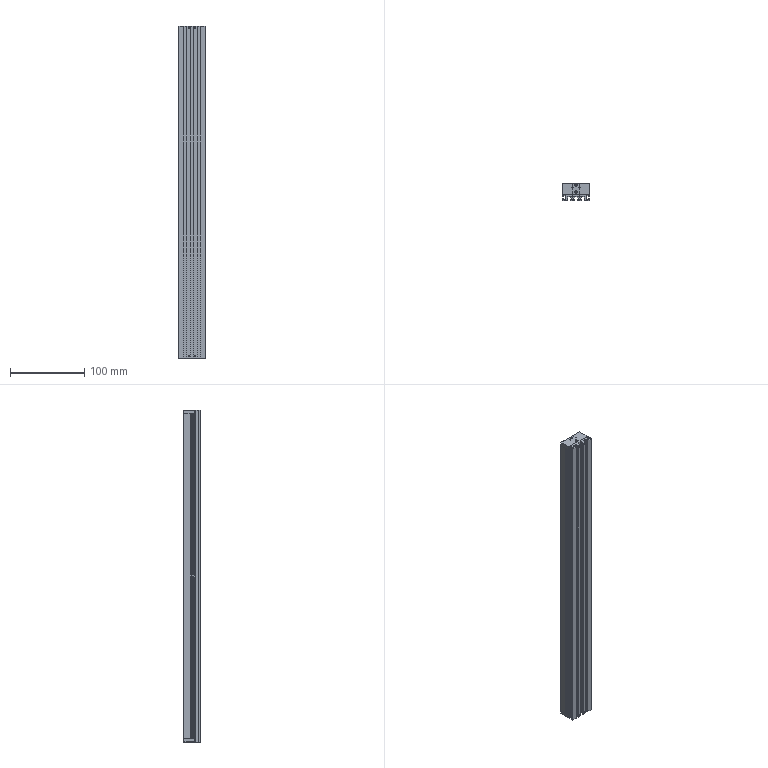Part | SolidWorks | 21 solids | 2933 faces | box 36 x 22.6 x 446 mm | volume 126686 mm3 | spline 1080 | plane 805 | cylinder 798 | cone 250 | commonest cylinder face diameters 2 x434 1.9 x216 0.2 x90 0.6 x24 1.6 x10 2.2 x8